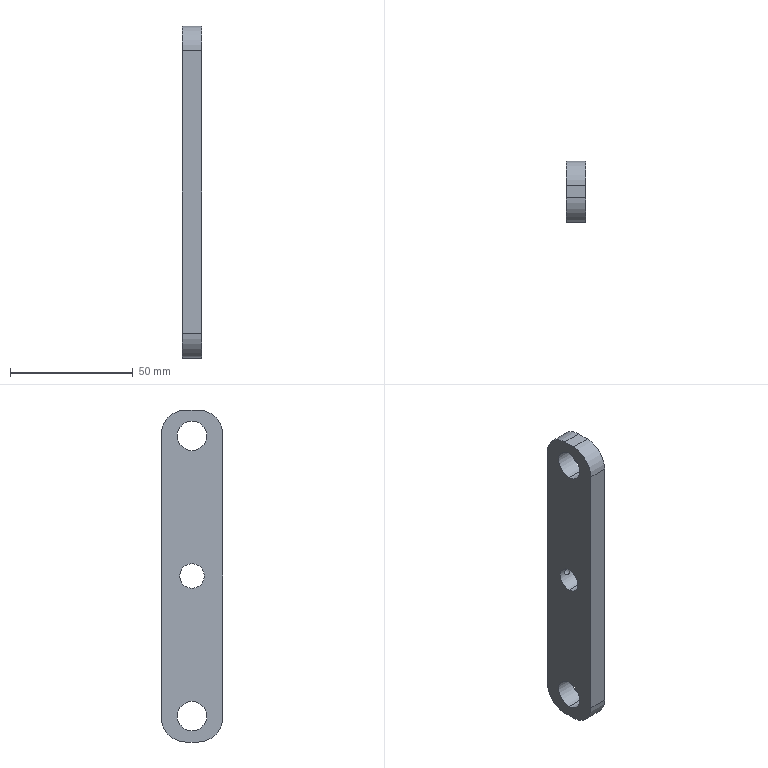Part | STEP file | 04-03 Suction nozzle link | 1 solid | 18 faces | box 8 x 25 x 135 mm | volume 23811 mm3 | cylinder 12 | plane 6 | commonest cylinder face diameters 12 x4 20 x4 3.3 x2 10 x2